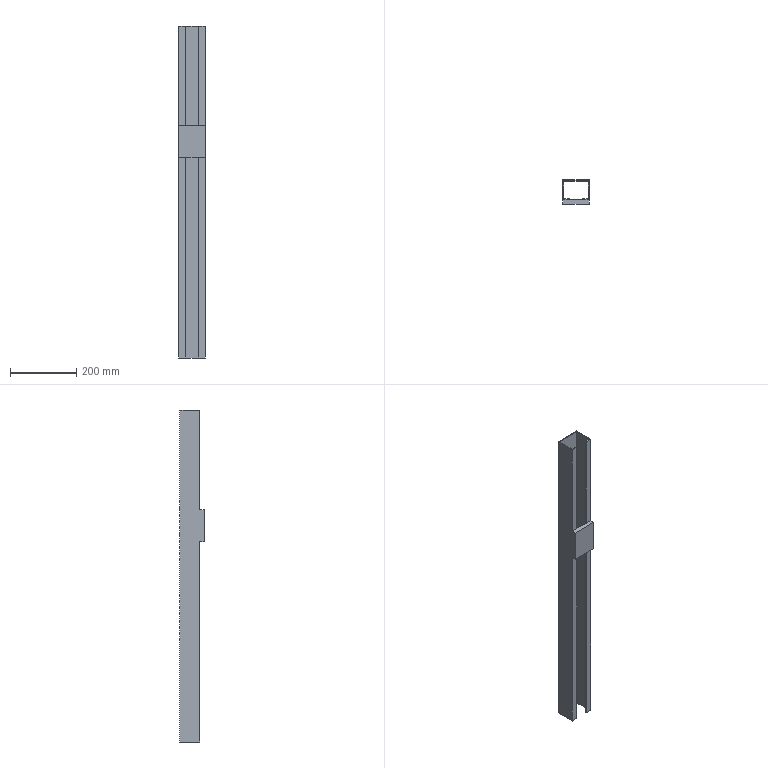Part | STEP file | 1 solid | 20 faces | box 80 x 73 x 1000 mm | volume 784880 mm3 | plane 20